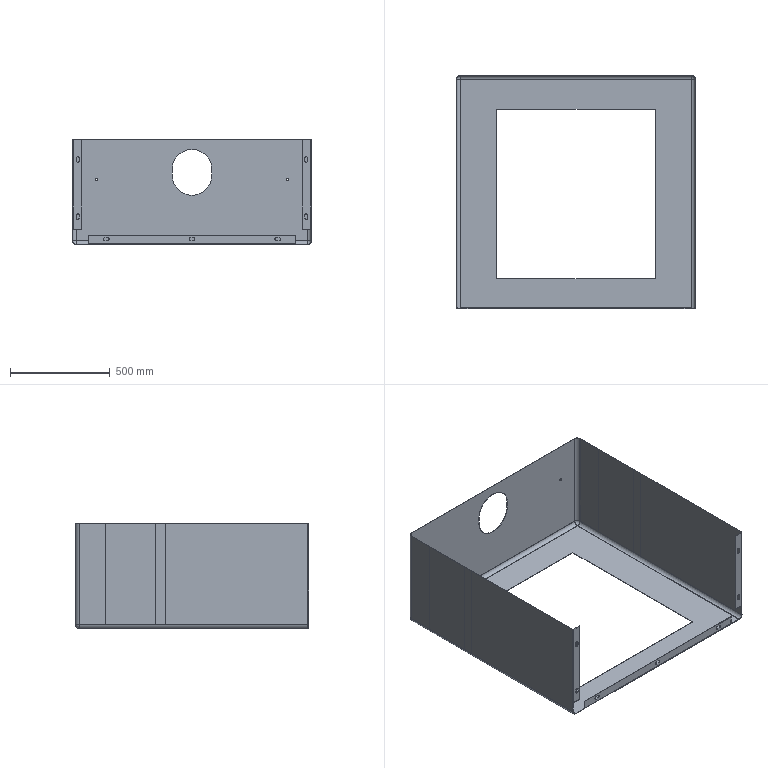Part | SolidWorks | features ICE 9, Fillet 4, LPattern 3, MirrorPattern 3, Extrusion 1, Shell 1 | 1 solid | 105 faces | box 1200 x 1170 x 527 mm | volume 5175590 mm3 | plane 58 | cylinder 41 | sphere 4 | torus 2 | commonest cylinder face diameters 14 x18 36 x5 40 x5 8 x4 12 x4 200 x3